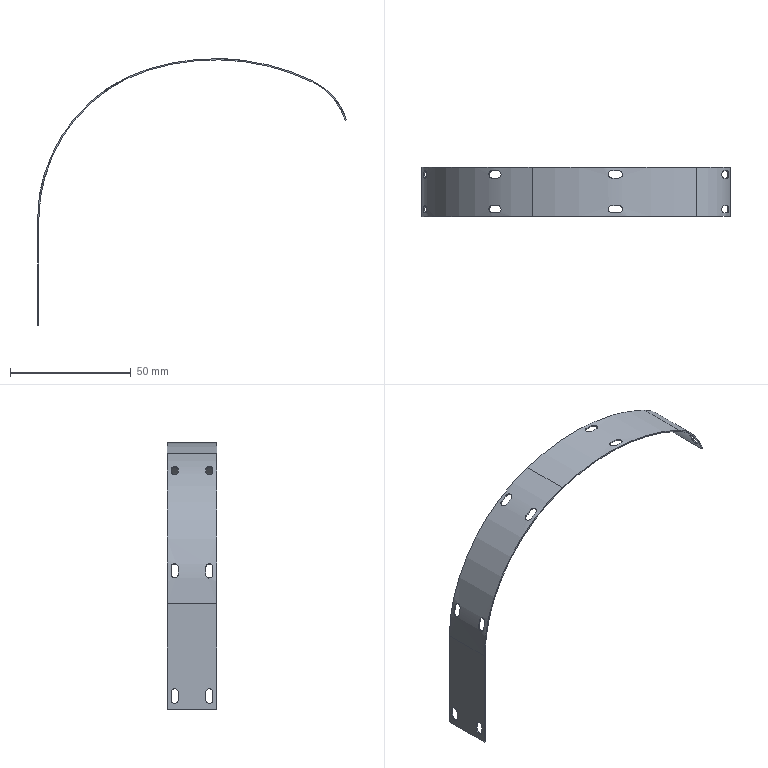Part | SolidWorks | features ICE 6, CurvePattern 1, Extrusion 1 | 1 solid | 62 faces | box 127.94 x 20.4 x 110.5 mm | volume 2142 mm3 | cylinder 36 | plane 26 | commonest cylinder face diameters 3 x30 53 x1 54 x1 130 x1 131 x1 184.469 x1